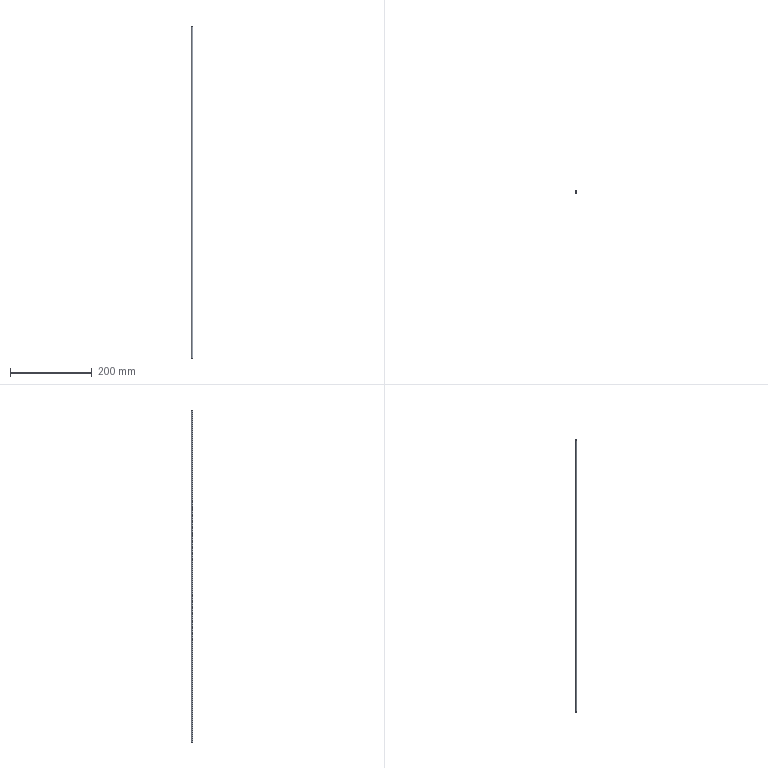Part | SolidWorks | features Extrusion 1 | 1 solid | 4 faces | box 4 x 4 x 810 mm | volume 10179 mm3 | cylinder 2 | plane 2 | commonest cylinder face diameters 4 x2
STEP:
#1=CARTESIAN_POINT('',(2.,0.,810.));
#2=VERTEX_POINT('',#1);
#3=CARTESIAN_POINT('',(-2.,0.,810.));
#4=VERTEX_POINT('',#3);
#5=CARTESIAN_POINT('',(0.,0.,810.));
#6=DIRECTION('',(0.,0.,1.));
#7=DIRECTION('',(1.,0.,0.));
#8=AXIS2_PLACEMENT_3D('',#5,#6,#7);
#9=CIRCLE('',#8,2.);
#10=EDGE_CURVE('',#2,#4,#9,.T.);
#11=ORIENTED_EDGE('',*,*,#10,.F.);
#12=CARTESIAN_POINT('',(2.,0.,0.));
#13=VERTEX_POINT('',#12);
#14=CARTESIAN_POINT('',(2.,0.,810.));
#15=DIRECTION('',(0.,0.,-1.));
#16=VECTOR('',#15,1000.);
#17=LINE('',#14,#16);
#18=EDGE_CURVE('',#2,#13,#17,.T.);
#19=ORIENTED_EDGE('',*,*,#18,.T.);
#20=CARTESIAN_POINT('',(-2.,0.,0.));
#21=VERTEX_POINT('',#20);
#22=CARTESIAN_POINT('',(0.,0.,0.));
#23=DIRECTION('',(0.,0.,1.));
#24=DIRECTION('',(1.,0.,0.));
#25=AXIS2_PLACEMENT_3D('',#22,#23,#24);
#26=CIRCLE('',#25,2.);
#27=EDGE_CURVE('',#13,#21,#26,.T.);
#28=ORIENTED_EDGE('',*,*,#27,.T.);
#29=CARTESIAN_POINT('',(-2.,0.,810.));
#30=DIRECTION('',(0.,0.,-1.));
#31=VECTOR('',#30,1000.);
#32=LINE('',#29,#31);
#33=EDGE_CURVE('',#4,#21,#32,.T.);
#34=ORIENTED_EDGE('',*,*,#33,.F.);
#35=EDGE_LOOP('',(#11,#19,#28,#34));
#36=FACE_OUTER_BOUND('',#35,.T.);
#37=CARTESIAN_POINT('',(0.,0.,810.));
#38=DIRECTION('',(0.,0.,-1.));
#39=DIRECTION('',(-1.,0.,0.));
#40=AXIS2_PLACEMENT_3D('',#37,#38,#39);
#41=CYLINDRICAL_SURFACE('',#40,2.);
#42=ADVANCED_FACE('',(#36),#41,.T.);
#43=ORIENTED_EDGE('',*,*,#18,.F.);
#44=CARTESIAN_POINT('',(0.,0.,810.));
#45=DIRECTION('',(0.,0.,1.));
#46=DIRECTION('',(1.,0.,0.));
#47=AXIS2_PLACEMENT_3D('',#44,#45,#46);
#48=CIRCLE('',#47,2.);
#49=EDGE_CURVE('',#4,#2,#48,.T.);
#50=ORIENTED_EDGE('',*,*,#49,.F.);
#51=ORIENTED_EDGE('',*,*,#33,.T.);
#52=CARTESIAN_POINT('',(0.,0.,0.));
#53=DIRECTION('',(0.,0.,1.));
#54=DIRECTION('',(1.,0.,0.));
#55=AXIS2_PLACEMENT_3D('',#52,#53,#54);
#56=CIRCLE('',#55,2.);
#57=EDGE_CURVE('',#21,#13,#56,.T.);
#58=ORIENTED_EDGE('',*,*,#57,.T.);
#59=EDGE_LOOP('',(#43,#50,#51,#58));
#60=FACE_OUTER_BOUND('',#59,.T.);
#61=CARTESIAN_POINT('',(0.,0.,810.));
#62=DIRECTION('',(0.,0.,-1.));
#63=DIRECTION('',(-1.,0.,0.));
#64=AXIS2_PLACEMENT_3D('',#61,#62,#63);
#65=CYLINDRICAL_SURFACE('',#64,2.);
#66=ADVANCED_FACE('',(#60),#65,.T.);
#67=ORIENTED_EDGE('',*,*,#49,.T.);
#68=ORIENTED_EDGE('',*,*,#10,.T.);
#69=EDGE_LOOP('',(#67,#68));
#70=FACE_OUTER_BOUND('',#69,.T.);
#71=CARTESIAN_POINT('',(0.,0.,810.));
#72=DIRECTION('',(0.,0.,1.));
#73=DIRECTION('',(1.,0.,0.));
#74=AXIS2_PLACEMENT_3D('',#71,#72,#73);
#75=PLANE('',#74);
#76=ADVANCED_FACE('',(#70),#75,.T.);
#77=ORIENTED_EDGE('',*,*,#57,.F.);
#78=ORIENTED_EDGE('',*,*,#27,.F.);
#79=EDGE_LOOP('',(#77,#78));
#80=FACE_OUTER_BOUND('',#79,.T.);
#81=CARTESIAN_POINT('',(0.,0.,0.));
#82=DIRECTION('',(0.,0.,1.));
#83=DIRECTION('',(1.,0.,0.));
#84=AXIS2_PLACEMENT_3D('',#81,#82,#83);
#85=PLANE('',#84);
#86=ADVANCED_FACE('',(#80),#85,.F.);
#87=CLOSED_SHELL('',(#42,#66,#76,#86));
#88=MANIFOLD_SOLID_BREP('',#87);
#89=CARTESIAN_POINT('',(0.,0.,0.));
#90=DIRECTION('',(0.,0.,1.));
#91=DIRECTION('',(1.,0.,0.));
#92=AXIS2_PLACEMENT_3D('',#89,#90,#91);
#93=(LENGTH_UNIT()NAMED_UNIT(*)SI_UNIT(.MILLI.,.METRE.));
#94=UNCERTAINTY_MEASURE_WITH_UNIT(LENGTH_MEASURE(0.00001),#93,'','');
#95=(NAMED_UNIT(*)PLANE_ANGLE_UNIT()SI_UNIT($,.RADIAN.));
#96=(NAMED_UNIT(*)SI_UNIT($,.STERADIAN.)SOLID_ANGLE_UNIT());
#97=(GEOMETRIC_REPRESENTATION_CONTEXT(3)GLOBAL_UNCERTAINTY_ASSIGNED_CONTEXT((#94))GLOBAL_UNIT_ASSIGNED_CONTEXT((#93,#95,#96))REPRESENTATION_CONTEXT('',''));
#98=ADVANCED_BREP_SHAPE_REPRESENTATION('',(#88,#92),#97);